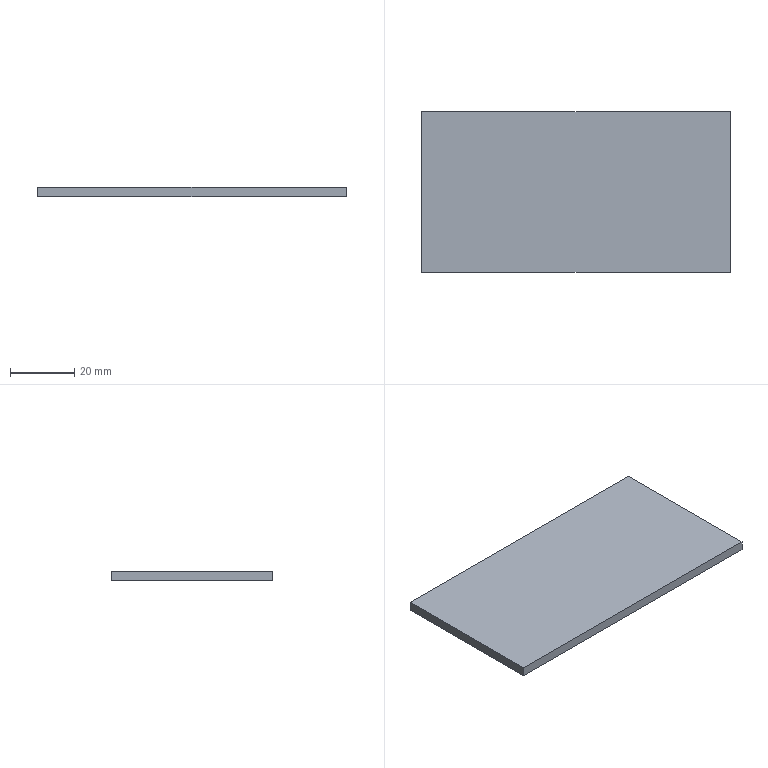Part | STEP file | SX-010-03 | 1 solid | 6 faces | box 96 x 50 x 3 mm | volume 14400 mm3 | plane 6
STEP:
#1=CARTESIAN_POINT('',(0.,0.,0.));
#2=DIRECTION('',(0.,0.,1.));
#3=DIRECTION('',(1.,0.,0.));
#4=AXIS2_PLACEMENT_3D('',#1,#2,#3);
#5=CARTESIAN_POINT('',(0.,50.,0.));
#6=VERTEX_POINT('',#5);
#7=CARTESIAN_POINT('',(0.,0.,0.));
#8=VERTEX_POINT('',#7);
#9=CARTESIAN_POINT('',(0.,0.,0.));
#10=DIRECTION('',(0.,-1.,0.));
#11=VECTOR('',#10,1.);
#12=LINE('',#9,#11);
#13=CARTESIAN_POINT('',(0.,0.,-3.));
#14=DIRECTION('',(-1.,0.,0.));
#15=DIRECTION('',(0.,-1.,0.));
#16=AXIS2_PLACEMENT_3D('',#13,#14,#15);
#17=PLANE('',#16);
#18=CARTESIAN_POINT('',(0.,3.));
#19=DIRECTION('',(1.,0.));
#20=VECTOR('',#19,1.);
#21=LINE('',#18,#20);
#22=(GEOMETRIC_REPRESENTATION_CONTEXT(2)PARAMETRIC_REPRESENTATION_CONTEXT()REPRESENTATION_CONTEXT('',''));
#23=DEFINITIONAL_REPRESENTATION('',(#21),#22);
#24=PCURVE('',#17,#23);
#25=CARTESIAN_POINT('',(0.,0.,0.));
#26=DIRECTION('',(0.,0.,-1.));
#27=DIRECTION('',(-1.,0.,0.));
#28=AXIS2_PLACEMENT_3D('',#25,#26,#27);
#29=PLANE('',#28);
#30=CARTESIAN_POINT('',(0.,0.));
#31=DIRECTION('',(0.,-1.));
#32=VECTOR('',#31,1.);
#33=LINE('',#30,#32);
#34=(GEOMETRIC_REPRESENTATION_CONTEXT(2)PARAMETRIC_REPRESENTATION_CONTEXT()REPRESENTATION_CONTEXT('',''));
#35=DEFINITIONAL_REPRESENTATION('',(#33),#34);
#36=PCURVE('',#29,#35);
#37=SURFACE_CURVE('',#12,(#24,#36),.PCURVE_S1.);
#38=EDGE_CURVE('',#6,#8,#37,.T.);
#39=ORIENTED_EDGE('',*,*,#38,.F.);
#40=CARTESIAN_POINT('',(0.,50.,-3.));
#41=VERTEX_POINT('',#40);
#42=CARTESIAN_POINT('',(0.,50.,-3.));
#43=DIRECTION('',(0.,0.,1.));
#44=VECTOR('',#43,1.);
#45=LINE('',#42,#44);
#46=CARTESIAN_POINT('',(-50.,0.));
#47=DIRECTION('',(0.,1.));
#48=VECTOR('',#47,1.);
#49=LINE('',#46,#48);
#50=(GEOMETRIC_REPRESENTATION_CONTEXT(2)PARAMETRIC_REPRESENTATION_CONTEXT()REPRESENTATION_CONTEXT('',''));
#51=DEFINITIONAL_REPRESENTATION('',(#49),#50);
#52=PCURVE('',#17,#51);
#53=CARTESIAN_POINT('',(0.,50.,-3.));
#54=DIRECTION('',(0.,1.,0.));
#55=DIRECTION('',(0.,0.,1.));
#56=AXIS2_PLACEMENT_3D('',#53,#54,#55);
#57=PLANE('',#56);
#58=CARTESIAN_POINT('',(0.,0.));
#59=DIRECTION('',(1.,0.));
#60=VECTOR('',#59,1.);
#61=LINE('',#58,#60);
#62=(GEOMETRIC_REPRESENTATION_CONTEXT(2)PARAMETRIC_REPRESENTATION_CONTEXT()REPRESENTATION_CONTEXT('',''));
#63=DEFINITIONAL_REPRESENTATION('',(#61),#62);
#64=PCURVE('',#57,#63);
#65=SURFACE_CURVE('',#45,(#52,#64),.PCURVE_S1.);
#66=EDGE_CURVE('',#41,#6,#65,.T.);
#67=ORIENTED_EDGE('',*,*,#66,.F.);
#68=CARTESIAN_POINT('',(0.,0.,-3.));
#69=VERTEX_POINT('',#68);
#70=CARTESIAN_POINT('',(0.,0.,-3.));
#71=DIRECTION('',(0.,-1.,0.));
#72=VECTOR('',#71,1.);
#73=LINE('',#70,#72);
#74=CARTESIAN_POINT('',(0.,0.));
#75=DIRECTION('',(1.,0.));
#76=VECTOR('',#75,1.);
#77=LINE('',#74,#76);
#78=(GEOMETRIC_REPRESENTATION_CONTEXT(2)PARAMETRIC_REPRESENTATION_CONTEXT()REPRESENTATION_CONTEXT('',''));
#79=DEFINITIONAL_REPRESENTATION('',(#77),#78);
#80=PCURVE('',#17,#79);
#81=CARTESIAN_POINT('',(0.,0.,-3.));
#82=DIRECTION('',(0.,0.,-1.));
#83=DIRECTION('',(-1.,0.,0.));
#84=AXIS2_PLACEMENT_3D('',#81,#82,#83);
#85=PLANE('',#84);
#86=CARTESIAN_POINT('',(0.,0.));
#87=DIRECTION('',(0.,-1.));
#88=VECTOR('',#87,1.);
#89=LINE('',#86,#88);
#90=(GEOMETRIC_REPRESENTATION_CONTEXT(2)PARAMETRIC_REPRESENTATION_CONTEXT()REPRESENTATION_CONTEXT('',''));
#91=DEFINITIONAL_REPRESENTATION('',(#89),#90);
#92=PCURVE('',#85,#91);
#93=SURFACE_CURVE('',#73,(#80,#92),.PCURVE_S1.);
#94=EDGE_CURVE('',#41,#69,#93,.T.);
#95=ORIENTED_EDGE('',*,*,#94,.T.);
#96=CARTESIAN_POINT('',(0.,0.,-3.));
#97=DIRECTION('',(0.,0.,1.));
#98=VECTOR('',#97,1.);
#99=LINE('',#96,#98);
#100=CARTESIAN_POINT('',(0.,0.));
#101=DIRECTION('',(0.,1.));
#102=VECTOR('',#101,1.);
#103=LINE('',#100,#102);
#104=(GEOMETRIC_REPRESENTATION_CONTEXT(2)PARAMETRIC_REPRESENTATION_CONTEXT()REPRESENTATION_CONTEXT('',''));
#105=DEFINITIONAL_REPRESENTATION('',(#103),#104);
#106=PCURVE('',#17,#105);
#107=CARTESIAN_POINT('',(0.,0.,-3.));
#108=DIRECTION('',(0.,-1.,0.));
#109=DIRECTION('',(0.,0.,-1.));
#110=AXIS2_PLACEMENT_3D('',#107,#108,#109);
#111=PLANE('',#110);
#112=CARTESIAN_POINT('',(0.,0.));
#113=DIRECTION('',(-1.,0.));
#114=VECTOR('',#113,1.);
#115=LINE('',#112,#114);
#116=(GEOMETRIC_REPRESENTATION_CONTEXT(2)PARAMETRIC_REPRESENTATION_CONTEXT()REPRESENTATION_CONTEXT('',''));
#117=DEFINITIONAL_REPRESENTATION('',(#115),#116);
#118=PCURVE('',#111,#117);
#119=SURFACE_CURVE('',#99,(#106,#118),.PCURVE_S1.);
#120=EDGE_CURVE('',#69,#8,#119,.T.);
#121=ORIENTED_EDGE('',*,*,#120,.T.);
#122=EDGE_LOOP('',(#39,#67,#95,#121));
#123=FACE_BOUND('',#122,.T.);
#124=ADVANCED_FACE('',(#123),#17,.T.);
#125=CARTESIAN_POINT('',(96.,50.,0.));
#126=VERTEX_POINT('',#125);
#127=CARTESIAN_POINT('',(0.,50.,0.));
#128=DIRECTION('',(-1.,0.,0.));
#129=VECTOR('',#128,1.);
#130=LINE('',#127,#129);
#131=CARTESIAN_POINT('',(3.,0.));
#132=DIRECTION('',(0.,-1.));
#133=VECTOR('',#132,1.);
#134=LINE('',#131,#133);
#135=(GEOMETRIC_REPRESENTATION_CONTEXT(2)PARAMETRIC_REPRESENTATION_CONTEXT()REPRESENTATION_CONTEXT('',''));
#136=DEFINITIONAL_REPRESENTATION('',(#134),#135);
#137=PCURVE('',#57,#136);
#138=CARTESIAN_POINT('',(0.,50.));
#139=DIRECTION('',(1.,0.));
#140=VECTOR('',#139,1.);
#141=LINE('',#138,#140);
#142=(GEOMETRIC_REPRESENTATION_CONTEXT(2)PARAMETRIC_REPRESENTATION_CONTEXT()REPRESENTATION_CONTEXT('',''));
#143=DEFINITIONAL_REPRESENTATION('',(#141),#142);
#144=PCURVE('',#29,#143);
#145=SURFACE_CURVE('',#130,(#137,#144),.PCURVE_S1.);
#146=EDGE_CURVE('',#126,#6,#145,.T.);
#147=ORIENTED_EDGE('',*,*,#146,.F.);
#148=CARTESIAN_POINT('',(96.,50.,-3.));
#149=VERTEX_POINT('',#148);
#150=CARTESIAN_POINT('',(96.,50.,-3.));
#151=DIRECTION('',(0.,0.,1.));
#152=VECTOR('',#151,1.);
#153=LINE('',#150,#152);
#154=CARTESIAN_POINT('',(0.,96.));
#155=DIRECTION('',(1.,0.));
#156=VECTOR('',#155,1.);
#157=LINE('',#154,#156);
#158=(GEOMETRIC_REPRESENTATION_CONTEXT(2)PARAMETRIC_REPRESENTATION_CONTEXT()REPRESENTATION_CONTEXT('',''));
#159=DEFINITIONAL_REPRESENTATION('',(#157),#158);
#160=PCURVE('',#57,#159);
#161=CARTESIAN_POINT('',(96.,0.,-3.));
#162=DIRECTION('',(1.,0.,0.));
#163=DIRECTION('',(0.,1.,0.));
#164=AXIS2_PLACEMENT_3D('',#161,#162,#163);
#165=PLANE('',#164);
#166=CARTESIAN_POINT('',(50.,0.));
#167=DIRECTION('',(0.,1.));
#168=VECTOR('',#167,1.);
#169=LINE('',#166,#168);
#170=(GEOMETRIC_REPRESENTATION_CONTEXT(2)PARAMETRIC_REPRESENTATION_CONTEXT()REPRESENTATION_CONTEXT('',''));
#171=DEFINITIONAL_REPRESENTATION('',(#169),#170);
#172=PCURVE('',#165,#171);
#173=SURFACE_CURVE('',#153,(#160,#172),.PCURVE_S1.);
#174=EDGE_CURVE('',#149,#126,#173,.T.);
#175=ORIENTED_EDGE('',*,*,#174,.F.);
#176=CARTESIAN_POINT('',(0.,50.,-3.));
#177=DIRECTION('',(-1.,0.,0.));
#178=VECTOR('',#177,1.);
#179=LINE('',#176,#178);
#180=CARTESIAN_POINT('',(0.,0.));
#181=DIRECTION('',(0.,-1.));
#182=VECTOR('',#181,1.);
#183=LINE('',#180,#182);
#184=(GEOMETRIC_REPRESENTATION_CONTEXT(2)PARAMETRIC_REPRESENTATION_CONTEXT()REPRESENTATION_CONTEXT('',''));
#185=DEFINITIONAL_REPRESENTATION('',(#183),#184);
#186=PCURVE('',#57,#185);
#187=CARTESIAN_POINT('',(0.,50.));
#188=DIRECTION('',(1.,0.));
#189=VECTOR('',#188,1.);
#190=LINE('',#187,#189);
#191=(GEOMETRIC_REPRESENTATION_CONTEXT(2)PARAMETRIC_REPRESENTATION_CONTEXT()REPRESENTATION_CONTEXT('',''));
#192=DEFINITIONAL_REPRESENTATION('',(#190),#191);
#193=PCURVE('',#85,#192);
#194=SURFACE_CURVE('',#179,(#186,#193),.PCURVE_S1.);
#195=EDGE_CURVE('',#149,#41,#194,.T.);
#196=ORIENTED_EDGE('',*,*,#195,.T.);
#197=ORIENTED_EDGE('',*,*,#66,.T.);
#198=EDGE_LOOP('',(#147,#175,#196,#197));
#199=FACE_BOUND('',#198,.T.);
#200=ADVANCED_FACE('',(#199),#57,.T.);
#201=CARTESIAN_POINT('',(96.,0.,0.));
#202=VERTEX_POINT('',#201);
#203=CARTESIAN_POINT('',(96.,0.,0.));
#204=DIRECTION('',(0.,1.,0.));
#205=VECTOR('',#204,1.);
#206=LINE('',#203,#205);
#207=CARTESIAN_POINT('',(0.,3.));
#208=DIRECTION('',(1.,0.));
#209=VECTOR('',#208,1.);
#210=LINE('',#207,#209);
#211=(GEOMETRIC_REPRESENTATION_CONTEXT(2)PARAMETRIC_REPRESENTATION_CONTEXT()REPRESENTATION_CONTEXT('',''));
#212=DEFINITIONAL_REPRESENTATION('',(#210),#211);
#213=PCURVE('',#165,#212);
#214=CARTESIAN_POINT('',(-96.,0.));
#215=DIRECTION('',(0.,1.));
#216=VECTOR('',#215,1.);
#217=LINE('',#214,#216);
#218=(GEOMETRIC_REPRESENTATION_CONTEXT(2)PARAMETRIC_REPRESENTATION_CONTEXT()REPRESENTATION_CONTEXT('',''));
#219=DEFINITIONAL_REPRESENTATION('',(#217),#218);
#220=PCURVE('',#29,#219);
#221=SURFACE_CURVE('',#206,(#213,#220),.PCURVE_S1.);
#222=EDGE_CURVE('',#202,#126,#221,.T.);
#223=ORIENTED_EDGE('',*,*,#222,.F.);
#224=CARTESIAN_POINT('',(96.,0.,-3.));
#225=VERTEX_POINT('',#224);
#226=CARTESIAN_POINT('',(96.,0.,-3.));
#227=DIRECTION('',(0.,0.,1.));
#228=VECTOR('',#227,1.);
#229=LINE('',#226,#228);
#230=CARTESIAN_POINT('',(0.,0.));
#231=DIRECTION('',(0.,1.));
#232=VECTOR('',#231,1.);
#233=LINE('',#230,#232);
#234=(GEOMETRIC_REPRESENTATION_CONTEXT(2)PARAMETRIC_REPRESENTATION_CONTEXT()REPRESENTATION_CONTEXT('',''));
#235=DEFINITIONAL_REPRESENTATION('',(#233),#234);
#236=PCURVE('',#165,#235);
#237=CARTESIAN_POINT('',(0.,96.));
#238=DIRECTION('',(-1.,0.));
#239=VECTOR('',#238,1.);
#240=LINE('',#237,#239);
#241=(GEOMETRIC_REPRESENTATION_CONTEXT(2)PARAMETRIC_REPRESENTATION_CONTEXT()REPRESENTATION_CONTEXT('',''));
#242=DEFINITIONAL_REPRESENTATION('',(#240),#241);
#243=PCURVE('',#111,#242);
#244=SURFACE_CURVE('',#229,(#236,#243),.PCURVE_S1.);
#245=EDGE_CURVE('',#225,#202,#244,.T.);
#246=ORIENTED_EDGE('',*,*,#245,.F.);
#247=CARTESIAN_POINT('',(96.,0.,-3.));
#248=DIRECTION('',(0.,1.,0.));
#249=VECTOR('',#248,1.);
#250=LINE('',#247,#249);
#251=CARTESIAN_POINT('',(0.,0.));
#252=DIRECTION('',(1.,0.));
#253=VECTOR('',#252,1.);
#254=LINE('',#251,#253);
#255=(GEOMETRIC_REPRESENTATION_CONTEXT(2)PARAMETRIC_REPRESENTATION_CONTEXT()REPRESENTATION_CONTEXT('',''));
#256=DEFINITIONAL_REPRESENTATION('',(#254),#255);
#257=PCURVE('',#165,#256);
#258=CARTESIAN_POINT('',(-96.,0.));
#259=DIRECTION('',(0.,1.));
#260=VECTOR('',#259,1.);
#261=LINE('',#258,#260);
#262=(GEOMETRIC_REPRESENTATION_CONTEXT(2)PARAMETRIC_REPRESENTATION_CONTEXT()REPRESENTATION_CONTEXT('',''));
#263=DEFINITIONAL_REPRESENTATION('',(#261),#262);
#264=PCURVE('',#85,#263);
#265=SURFACE_CURVE('',#250,(#257,#264),.PCURVE_S1.);
#266=EDGE_CURVE('',#225,#149,#265,.T.);
#267=ORIENTED_EDGE('',*,*,#266,.T.);
#268=ORIENTED_EDGE('',*,*,#174,.T.);
#269=EDGE_LOOP('',(#223,#246,#267,#268));
#270=FACE_BOUND('',#269,.T.);
#271=ADVANCED_FACE('',(#270),#165,.T.);
#272=CARTESIAN_POINT('',(0.,0.,0.));
#273=DIRECTION('',(1.,0.,0.));
#274=VECTOR('',#273,1.);
#275=LINE('',#272,#274);
#276=CARTESIAN_POINT('',(-3.,0.));
#277=DIRECTION('',(0.,1.));
#278=VECTOR('',#277,1.);
#279=LINE('',#276,#278);
#280=(GEOMETRIC_REPRESENTATION_CONTEXT(2)PARAMETRIC_REPRESENTATION_CONTEXT()REPRESENTATION_CONTEXT('',''));
#281=DEFINITIONAL_REPRESENTATION('',(#279),#280);
#282=PCURVE('',#111,#281);
#283=CARTESIAN_POINT('',(0.,0.));
#284=DIRECTION('',(-1.,0.));
#285=VECTOR('',#284,1.);
#286=LINE('',#283,#285);
#287=(GEOMETRIC_REPRESENTATION_CONTEXT(2)PARAMETRIC_REPRESENTATION_CONTEXT()REPRESENTATION_CONTEXT('',''));
#288=DEFINITIONAL_REPRESENTATION('',(#286),#287);
#289=PCURVE('',#29,#288);
#290=SURFACE_CURVE('',#275,(#282,#289),.PCURVE_S1.);
#291=EDGE_CURVE('',#8,#202,#290,.T.);
#292=ORIENTED_EDGE('',*,*,#291,.F.);
#293=ORIENTED_EDGE('',*,*,#120,.F.);
#294=CARTESIAN_POINT('',(0.,0.,-3.));
#295=DIRECTION('',(1.,0.,0.));
#296=VECTOR('',#295,1.);
#297=LINE('',#294,#296);
#298=CARTESIAN_POINT('',(0.,0.));
#299=DIRECTION('',(0.,1.));
#300=VECTOR('',#299,1.);
#301=LINE('',#298,#300);
#302=(GEOMETRIC_REPRESENTATION_CONTEXT(2)PARAMETRIC_REPRESENTATION_CONTEXT()REPRESENTATION_CONTEXT('',''));
#303=DEFINITIONAL_REPRESENTATION('',(#301),#302);
#304=PCURVE('',#111,#303);
#305=CARTESIAN_POINT('',(0.,0.));
#306=DIRECTION('',(-1.,0.));
#307=VECTOR('',#306,1.);
#308=LINE('',#305,#307);
#309=(GEOMETRIC_REPRESENTATION_CONTEXT(2)PARAMETRIC_REPRESENTATION_CONTEXT()REPRESENTATION_CONTEXT('',''));
#310=DEFINITIONAL_REPRESENTATION('',(#308),#309);
#311=PCURVE('',#85,#310);
#312=SURFACE_CURVE('',#297,(#304,#311),.PCURVE_S1.);
#313=EDGE_CURVE('',#69,#225,#312,.T.);
#314=ORIENTED_EDGE('',*,*,#313,.T.);
#315=ORIENTED_EDGE('',*,*,#245,.T.);
#316=EDGE_LOOP('',(#292,#293,#314,#315));
#317=FACE_BOUND('',#316,.T.);
#318=ADVANCED_FACE('',(#317),#111,.T.);
#319=ORIENTED_EDGE('',*,*,#94,.F.);
#320=ORIENTED_EDGE('',*,*,#195,.F.);
#321=ORIENTED_EDGE('',*,*,#266,.F.);
#322=ORIENTED_EDGE('',*,*,#313,.F.);
#323=EDGE_LOOP('',(#319,#320,#321,#322));
#324=FACE_BOUND('',#323,.T.);
#325=ADVANCED_FACE('',(#324),#85,.T.);
#326=ORIENTED_EDGE('',*,*,#38,.T.);
#327=ORIENTED_EDGE('',*,*,#291,.T.);
#328=ORIENTED_EDGE('',*,*,#222,.T.);
#329=ORIENTED_EDGE('',*,*,#146,.T.);
#330=EDGE_LOOP('',(#326,#327,#328,#329));
#331=FACE_BOUND('',#330,.T.);
#332=ADVANCED_FACE('',(#331),#29,.F.);
#333=CLOSED_SHELL('',(#124,#200,#271,#318,#325,#332));
#334=MANIFOLD_SOLID_BREP('',#333);
#335=(LENGTH_UNIT()NAMED_UNIT(*)SI_UNIT(.MILLI.,.METRE.));
#336=UNCERTAINTY_MEASURE_WITH_UNIT(LENGTH_MEASURE(0.0000001),#335,'','');
#337=(NAMED_UNIT(*)PLANE_ANGLE_UNIT()SI_UNIT($,.RADIAN.));
#338=(NAMED_UNIT(*)SI_UNIT($,.STERADIAN.)SOLID_ANGLE_UNIT());
#339=(GEOMETRIC_REPRESENTATION_CONTEXT(3)GLOBAL_UNCERTAINTY_ASSIGNED_CONTEXT((#336))GLOBAL_UNIT_ASSIGNED_CONTEXT((#335,#337,#338))REPRESENTATION_CONTEXT('',''));
#340=ADVANCED_BREP_SHAPE_REPRESENTATION('',(#4,#334),#339);